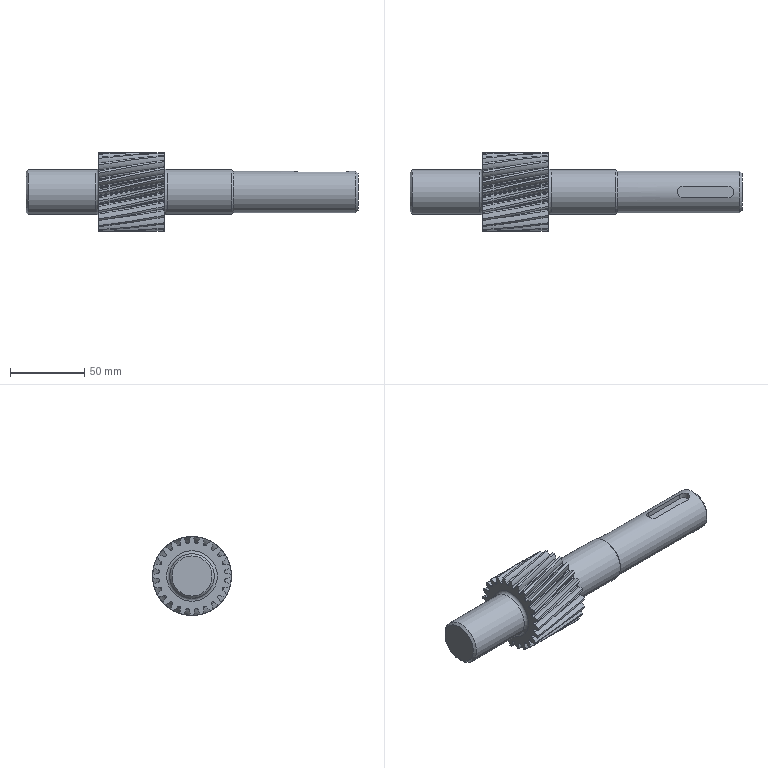Part | NX | features BREP 24, META 24, DATUM_CSYS 3, SKETCH 2, BLEND 1, CHAMFER 1, CYLINDER 1, EXTRUDE 1, FSET 1, SWP104 1 | 1 solid | 161 faces | box 223.5 x 53.091 x 53.091 mm | volume 200222 mm3 | spline 120 | cylinder 29 | plane 7 | torus 3 | cone 2 | commonest cylinder face diameters 44.091 x24 8 x2 30 x2 28 x1